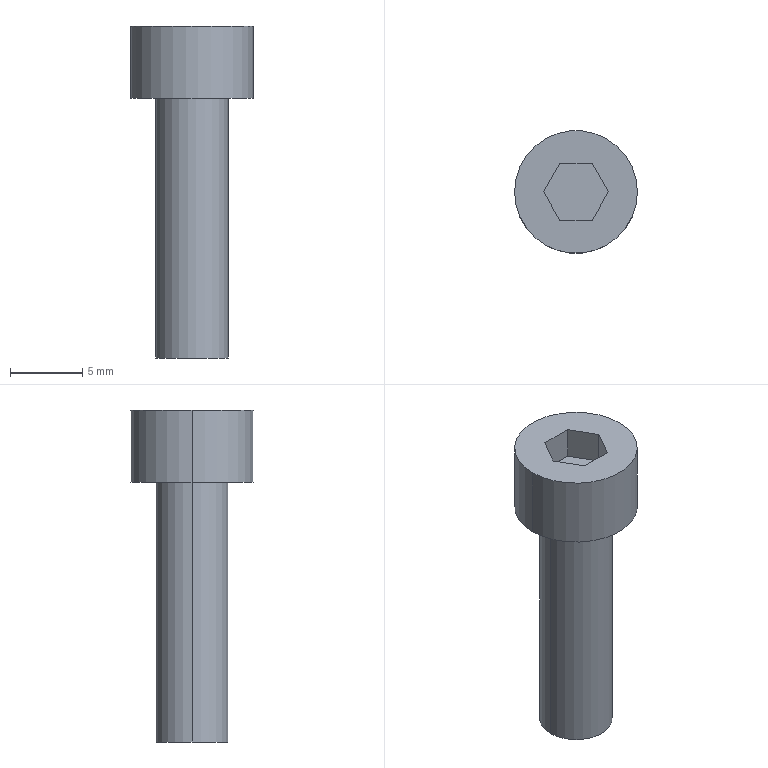Part | SolidWorks | features BaseBody 1 | 1 solid | 14 faces | box 8.5 x 8.5 x 23 mm | volume 607.561 mm3 | plane 10 | cylinder 4 | commonest cylinder face diameters 5 x2 8.5 x2
STEP:
#1=CARTESIAN_POINT('',(2.5,0.,-18.));
#2=VERTEX_POINT('',#1);
#3=CARTESIAN_POINT('',(-2.5,0.,-18.));
#4=VERTEX_POINT('',#3);
#5=CARTESIAN_POINT('',(0.,0.,-18.));
#6=DIRECTION('',(0.,0.,1.));
#7=DIRECTION('',(1.,0.,0.));
#8=AXIS2_PLACEMENT_3D('',#5,#6,#7);
#9=CIRCLE('',#8,2.5);
#10=EDGE_CURVE('',#2,#4,#9,.T.);
#11=ORIENTED_EDGE('',*,*,#10,.T.);
#12=CARTESIAN_POINT('',(-2.5,0.,0.));
#13=VERTEX_POINT('',#12);
#14=CARTESIAN_POINT('',(-2.5,0.,-18.));
#15=DIRECTION('',(0.,0.,1.));
#16=VECTOR('',#15,1000.);
#17=LINE('',#14,#16);
#18=EDGE_CURVE('',#4,#13,#17,.T.);
#19=ORIENTED_EDGE('',*,*,#18,.T.);
#20=CARTESIAN_POINT('',(2.5,0.,0.));
#21=VERTEX_POINT('',#20);
#22=CARTESIAN_POINT('',(0.,0.,0.));
#23=DIRECTION('',(0.,0.,-1.));
#24=DIRECTION('',(1.,0.,0.));
#25=AXIS2_PLACEMENT_3D('',#22,#23,#24);
#26=CIRCLE('',#25,2.5);
#27=EDGE_CURVE('',#13,#21,#26,.T.);
#28=ORIENTED_EDGE('',*,*,#27,.T.);
#29=CARTESIAN_POINT('',(2.5,0.,-18.));
#30=DIRECTION('',(0.,0.,1.));
#31=VECTOR('',#30,1000.);
#32=LINE('',#29,#31);
#33=EDGE_CURVE('',#2,#21,#32,.T.);
#34=ORIENTED_EDGE('',*,*,#33,.F.);
#35=EDGE_LOOP('',(#11,#19,#28,#34));
#36=FACE_OUTER_BOUND('',#35,.T.);
#37=CARTESIAN_POINT('',(0.,0.,-18.));
#38=DIRECTION('',(0.,0.,1.));
#39=DIRECTION('',(1.,0.,0.));
#40=AXIS2_PLACEMENT_3D('',#37,#38,#39);
#41=CYLINDRICAL_SURFACE('',#40,2.5);
#42=ADVANCED_FACE('',(#36),#41,.T.);
#43=CARTESIAN_POINT('',(4.25,0.,0.));
#44=VERTEX_POINT('',#43);
#45=CARTESIAN_POINT('',(-4.25,0.,0.));
#46=VERTEX_POINT('',#45);
#47=CARTESIAN_POINT('',(0.,0.,0.));
#48=DIRECTION('',(0.,0.,1.));
#49=DIRECTION('',(1.,0.,0.));
#50=AXIS2_PLACEMENT_3D('',#47,#48,#49);
#51=CIRCLE('',#50,4.25);
#52=EDGE_CURVE('',#44,#46,#51,.T.);
#53=ORIENTED_EDGE('',*,*,#52,.T.);
#54=CARTESIAN_POINT('',(-4.25,0.,5.));
#55=VERTEX_POINT('',#54);
#56=CARTESIAN_POINT('',(-4.25,0.,0.));
#57=DIRECTION('',(0.,0.,1.));
#58=VECTOR('',#57,1000.);
#59=LINE('',#56,#58);
#60=EDGE_CURVE('',#46,#55,#59,.T.);
#61=ORIENTED_EDGE('',*,*,#60,.T.);
#62=CARTESIAN_POINT('',(4.25,0.,5.));
#63=VERTEX_POINT('',#62);
#64=CARTESIAN_POINT('',(0.,0.,5.));
#65=DIRECTION('',(0.,0.,-1.));
#66=DIRECTION('',(1.,0.,0.));
#67=AXIS2_PLACEMENT_3D('',#64,#65,#66);
#68=CIRCLE('',#67,4.25);
#69=EDGE_CURVE('',#55,#63,#68,.T.);
#70=ORIENTED_EDGE('',*,*,#69,.T.);
#71=CARTESIAN_POINT('',(4.25,0.,0.));
#72=DIRECTION('',(0.,0.,1.));
#73=VECTOR('',#72,1000.);
#74=LINE('',#71,#73);
#75=EDGE_CURVE('',#44,#63,#74,.T.);
#76=ORIENTED_EDGE('',*,*,#75,.F.);
#77=EDGE_LOOP('',(#53,#61,#70,#76));
#78=FACE_OUTER_BOUND('',#77,.T.);
#79=CARTESIAN_POINT('',(0.,0.,0.));
#80=DIRECTION('',(0.,0.,1.));
#81=DIRECTION('',(1.,0.,0.));
#82=AXIS2_PLACEMENT_3D('',#79,#80,#81);
#83=CYLINDRICAL_SURFACE('',#82,4.25);
#84=ADVANCED_FACE('',(#78),#83,.T.);
#85=ORIENTED_EDGE('',*,*,#18,.F.);
#86=CARTESIAN_POINT('',(0.,0.,-18.));
#87=DIRECTION('',(0.,0.,1.));
#88=DIRECTION('',(1.,0.,0.));
#89=AXIS2_PLACEMENT_3D('',#86,#87,#88);
#90=CIRCLE('',#89,2.5);
#91=EDGE_CURVE('',#4,#2,#90,.T.);
#92=ORIENTED_EDGE('',*,*,#91,.T.);
#93=ORIENTED_EDGE('',*,*,#33,.T.);
#94=CARTESIAN_POINT('',(0.,0.,0.));
#95=DIRECTION('',(0.,0.,-1.));
#96=DIRECTION('',(1.,0.,0.));
#97=AXIS2_PLACEMENT_3D('',#94,#95,#96);
#98=CIRCLE('',#97,2.5);
#99=EDGE_CURVE('',#21,#13,#98,.T.);
#100=ORIENTED_EDGE('',*,*,#99,.T.);
#101=EDGE_LOOP('',(#85,#92,#93,#100));
#102=FACE_OUTER_BOUND('',#101,.T.);
#103=CARTESIAN_POINT('',(0.,0.,-18.));
#104=DIRECTION('',(0.,0.,1.));
#105=DIRECTION('',(1.,0.,0.));
#106=AXIS2_PLACEMENT_3D('',#103,#104,#105);
#107=CYLINDRICAL_SURFACE('',#106,2.5);
#108=ADVANCED_FACE('',(#102),#107,.T.);
#109=ORIENTED_EDGE('',*,*,#10,.F.);
#110=ORIENTED_EDGE('',*,*,#91,.F.);
#111=EDGE_LOOP('',(#109,#110));
#112=FACE_OUTER_BOUND('',#111,.T.);
#113=CARTESIAN_POINT('',(0.,0.,-18.));
#114=DIRECTION('',(0.,0.,1.));
#115=DIRECTION('',(1.,0.,0.));
#116=AXIS2_PLACEMENT_3D('',#113,#114,#115);
#117=PLANE('',#116);
#118=ADVANCED_FACE('',(#112),#117,.F.);
#119=ORIENTED_EDGE('',*,*,#99,.F.);
#120=ORIENTED_EDGE('',*,*,#27,.F.);
#121=EDGE_LOOP('',(#119,#120));
#122=FACE_BOUND('',#121,.T.);
#123=ORIENTED_EDGE('',*,*,#52,.F.);
#124=CARTESIAN_POINT('',(0.,0.,0.));
#125=DIRECTION('',(0.,0.,1.));
#126=DIRECTION('',(1.,0.,0.));
#127=AXIS2_PLACEMENT_3D('',#124,#125,#126);
#128=CIRCLE('',#127,4.25);
#129=EDGE_CURVE('',#46,#44,#128,.T.);
#130=ORIENTED_EDGE('',*,*,#129,.F.);
#131=EDGE_LOOP('',(#123,#130));
#132=FACE_OUTER_BOUND('',#131,.T.);
#133=CARTESIAN_POINT('',(0.,0.,0.));
#134=DIRECTION('',(0.,0.,1.));
#135=DIRECTION('',(1.,0.,0.));
#136=AXIS2_PLACEMENT_3D('',#133,#134,#135);
#137=PLANE('',#136);
#138=ADVANCED_FACE('',(#122,#132),#137,.F.);
#139=ORIENTED_EDGE('',*,*,#60,.F.);
#140=ORIENTED_EDGE('',*,*,#129,.T.);
#141=ORIENTED_EDGE('',*,*,#75,.T.);
#142=CARTESIAN_POINT('',(0.,0.,5.));
#143=DIRECTION('',(0.,0.,-1.));
#144=DIRECTION('',(1.,0.,0.));
#145=AXIS2_PLACEMENT_3D('',#142,#143,#144);
#146=CIRCLE('',#145,4.25);
#147=EDGE_CURVE('',#63,#55,#146,.T.);
#148=ORIENTED_EDGE('',*,*,#147,.T.);
#149=EDGE_LOOP('',(#139,#140,#141,#148));
#150=FACE_OUTER_BOUND('',#149,.T.);
#151=CARTESIAN_POINT('',(0.,0.,0.));
#152=DIRECTION('',(0.,0.,1.));
#153=DIRECTION('',(1.,0.,0.));
#154=AXIS2_PLACEMENT_3D('',#151,#152,#153);
#155=CYLINDRICAL_SURFACE('',#154,4.25);
#156=ADVANCED_FACE('',(#150),#155,.T.);
#157=CARTESIAN_POINT('',(-1.125,-1.949,5.));
#158=VERTEX_POINT('',#157);
#159=CARTESIAN_POINT('',(-2.25,0.,5.));
#160=VERTEX_POINT('',#159);
#161=CARTESIAN_POINT('',(-1.125,-1.949,5.));
#162=DIRECTION('',(-0.5,0.866,0.));
#163=VECTOR('',#162,1000.);
#164=LINE('',#161,#163);
#165=EDGE_CURVE('',#158,#160,#164,.T.);
#166=ORIENTED_EDGE('',*,*,#165,.T.);
#167=CARTESIAN_POINT('',(-1.125,1.949,5.));
#168=VERTEX_POINT('',#167);
#169=CARTESIAN_POINT('',(-2.25,0.,5.));
#170=DIRECTION('',(0.5,0.866,0.));
#171=VECTOR('',#170,1000.);
#172=LINE('',#169,#171);
#173=EDGE_CURVE('',#160,#168,#172,.T.);
#174=ORIENTED_EDGE('',*,*,#173,.T.);
#175=CARTESIAN_POINT('',(1.125,1.949,5.));
#176=VERTEX_POINT('',#175);
#177=CARTESIAN_POINT('',(0.,1.949,5.));
#178=DIRECTION('',(1.,0.,0.));
#179=VECTOR('',#178,1000.);
#180=LINE('',#177,#179);
#181=EDGE_CURVE('',#168,#176,#180,.T.);
#182=ORIENTED_EDGE('',*,*,#181,.T.);
#183=CARTESIAN_POINT('',(2.25,0.,5.));
#184=VERTEX_POINT('',#183);
#185=CARTESIAN_POINT('',(1.125,1.949,5.));
#186=DIRECTION('',(0.5,-0.866,0.));
#187=VECTOR('',#186,1000.);
#188=LINE('',#185,#187);
#189=EDGE_CURVE('',#176,#184,#188,.T.);
#190=ORIENTED_EDGE('',*,*,#189,.T.);
#191=CARTESIAN_POINT('',(1.125,-1.949,5.));
#192=VERTEX_POINT('',#191);
#193=CARTESIAN_POINT('',(2.25,0.,5.));
#194=DIRECTION('',(-0.5,-0.866,0.));
#195=VECTOR('',#194,1000.);
#196=LINE('',#193,#195);
#197=EDGE_CURVE('',#184,#192,#196,.T.);
#198=ORIENTED_EDGE('',*,*,#197,.T.);
#199=CARTESIAN_POINT('',(0.,-1.949,5.));
#200=DIRECTION('',(-1.,0.,0.));
#201=VECTOR('',#200,1000.);
#202=LINE('',#199,#201);
#203=EDGE_CURVE('',#192,#158,#202,.T.);
#204=ORIENTED_EDGE('',*,*,#203,.T.);
#205=EDGE_LOOP('',(#166,#174,#182,#190,#198,#204));
#206=FACE_BOUND('',#205,.T.);
#207=ORIENTED_EDGE('',*,*,#147,.F.);
#208=ORIENTED_EDGE('',*,*,#69,.F.);
#209=EDGE_LOOP('',(#207,#208));
#210=FACE_OUTER_BOUND('',#209,.T.);
#211=CARTESIAN_POINT('',(0.,0.,5.));
#212=DIRECTION('',(0.,0.,1.));
#213=DIRECTION('',(1.,0.,0.));
#214=AXIS2_PLACEMENT_3D('',#211,#212,#213);
#215=PLANE('',#214);
#216=ADVANCED_FACE('',(#206,#210),#215,.T.);
#217=ORIENTED_EDGE('',*,*,#173,.F.);
#218=CARTESIAN_POINT('',(-2.25,0.,2.75));
#219=VERTEX_POINT('',#218);
#220=CARTESIAN_POINT('',(-2.25,0.,2.75));
#221=DIRECTION('',(0.,0.,-1.));
#222=VECTOR('',#221,1000.);
#223=LINE('',#220,#222);
#224=EDGE_CURVE('',#160,#219,#223,.T.);
#225=ORIENTED_EDGE('',*,*,#224,.T.);
#226=CARTESIAN_POINT('',(-1.125,1.949,2.75));
#227=VERTEX_POINT('',#226);
#228=CARTESIAN_POINT('',(-1.125,1.949,2.75));
#229=DIRECTION('',(0.5,0.866,0.));
#230=VECTOR('',#229,1000.);
#231=LINE('',#228,#230);
#232=EDGE_CURVE('',#219,#227,#231,.T.);
#233=ORIENTED_EDGE('',*,*,#232,.T.);
#234=CARTESIAN_POINT('',(-1.125,1.949,2.75));
#235=DIRECTION('',(0.,0.,1.));
#236=VECTOR('',#235,1000.);
#237=LINE('',#234,#236);
#238=EDGE_CURVE('',#227,#168,#237,.T.);
#239=ORIENTED_EDGE('',*,*,#238,.T.);
#240=EDGE_LOOP('',(#217,#225,#233,#239));
#241=FACE_OUTER_BOUND('',#240,.T.);
#242=CARTESIAN_POINT('',(-1.125,1.949,2.75));
#243=DIRECTION('',(0.866,-0.5,0.));
#244=DIRECTION('',(0.5,0.866,0.));
#245=AXIS2_PLACEMENT_3D('',#242,#243,#244);
#246=PLANE('',#245);
#247=ADVANCED_FACE('',(#241),#246,.T.);
#248=ORIENTED_EDGE('',*,*,#165,.F.);
#249=CARTESIAN_POINT('',(-1.125,-1.949,2.75));
#250=VERTEX_POINT('',#249);
#251=CARTESIAN_POINT('',(-1.125,-1.949,2.75));
#252=DIRECTION('',(0.,0.,-1.));
#253=VECTOR('',#252,1000.);
#254=LINE('',#251,#253);
#255=EDGE_CURVE('',#158,#250,#254,.T.);
#256=ORIENTED_EDGE('',*,*,#255,.T.);
#257=CARTESIAN_POINT('',(-2.25,0.,2.75));
#258=DIRECTION('',(-0.5,0.866,0.));
#259=VECTOR('',#258,1000.);
#260=LINE('',#257,#259);
#261=EDGE_CURVE('',#250,#219,#260,.T.);
#262=ORIENTED_EDGE('',*,*,#261,.T.);
#263=ORIENTED_EDGE('',*,*,#224,.F.);
#264=EDGE_LOOP('',(#248,#256,#262,#263));
#265=FACE_OUTER_BOUND('',#264,.T.);
#266=CARTESIAN_POINT('',(-2.25,0.,2.75));
#267=DIRECTION('',(0.866,0.5,0.));
#268=DIRECTION('',(-0.5,0.866,0.));
#269=AXIS2_PLACEMENT_3D('',#266,#267,#268);
#270=PLANE('',#269);
#271=ADVANCED_FACE('',(#265),#270,.T.);
#272=ORIENTED_EDGE('',*,*,#203,.F.);
#273=CARTESIAN_POINT('',(1.125,-1.949,2.75));
#274=VERTEX_POINT('',#273);
#275=CARTESIAN_POINT('',(1.125,-1.949,2.75));
#276=DIRECTION('',(0.,0.,-1.));
#277=VECTOR('',#276,1000.);
#278=LINE('',#275,#277);
#279=EDGE_CURVE('',#192,#274,#278,.T.);
#280=ORIENTED_EDGE('',*,*,#279,.T.);
#281=CARTESIAN_POINT('',(-1.125,-1.949,2.75));
#282=DIRECTION('',(-1.,0.,0.));
#283=VECTOR('',#282,1000.);
#284=LINE('',#281,#283);
#285=EDGE_CURVE('',#274,#250,#284,.T.);
#286=ORIENTED_EDGE('',*,*,#285,.T.);
#287=ORIENTED_EDGE('',*,*,#255,.F.);
#288=EDGE_LOOP('',(#272,#280,#286,#287));
#289=FACE_OUTER_BOUND('',#288,.T.);
#290=CARTESIAN_POINT('',(-1.125,-1.949,2.75));
#291=DIRECTION('',(0.,1.,0.));
#292=DIRECTION('',(-1.,0.,0.));
#293=AXIS2_PLACEMENT_3D('',#290,#291,#292);
#294=PLANE('',#293);
#295=ADVANCED_FACE('',(#289),#294,.T.);
#296=ORIENTED_EDGE('',*,*,#197,.F.);
#297=CARTESIAN_POINT('',(2.25,0.,2.75));
#298=VERTEX_POINT('',#297);
#299=CARTESIAN_POINT('',(2.25,0.,2.75));
#300=DIRECTION('',(0.,0.,-1.));
#301=VECTOR('',#300,1000.);
#302=LINE('',#299,#301);
#303=EDGE_CURVE('',#184,#298,#302,.T.);
#304=ORIENTED_EDGE('',*,*,#303,.T.);
#305=CARTESIAN_POINT('',(1.125,-1.949,2.75));
#306=DIRECTION('',(-0.5,-0.866,0.));
#307=VECTOR('',#306,1000.);
#308=LINE('',#305,#307);
#309=EDGE_CURVE('',#298,#274,#308,.T.);
#310=ORIENTED_EDGE('',*,*,#309,.T.);
#311=ORIENTED_EDGE('',*,*,#279,.F.);
#312=EDGE_LOOP('',(#296,#304,#310,#311));
#313=FACE_OUTER_BOUND('',#312,.T.);
#314=CARTESIAN_POINT('',(1.125,-1.949,2.75));
#315=DIRECTION('',(-0.866,0.5,0.));
#316=DIRECTION('',(-0.5,-0.866,0.));
#317=AXIS2_PLACEMENT_3D('',#314,#315,#316);
#318=PLANE('',#317);
#319=ADVANCED_FACE('',(#313),#318,.T.);
#320=ORIENTED_EDGE('',*,*,#189,.F.);
#321=CARTESIAN_POINT('',(1.125,1.949,2.75));
#322=VERTEX_POINT('',#321);
#323=CARTESIAN_POINT('',(1.125,1.949,2.75));
#324=DIRECTION('',(0.,0.,-1.));
#325=VECTOR('',#324,1000.);
#326=LINE('',#323,#325);
#327=EDGE_CURVE('',#176,#322,#326,.T.);
#328=ORIENTED_EDGE('',*,*,#327,.T.);
#329=CARTESIAN_POINT('',(2.25,0.,2.75));
#330=DIRECTION('',(0.5,-0.866,0.));
#331=VECTOR('',#330,1000.);
#332=LINE('',#329,#331);
#333=EDGE_CURVE('',#322,#298,#332,.T.);
#334=ORIENTED_EDGE('',*,*,#333,.T.);
#335=ORIENTED_EDGE('',*,*,#303,.F.);
#336=EDGE_LOOP('',(#320,#328,#334,#335));
#337=FACE_OUTER_BOUND('',#336,.T.);
#338=CARTESIAN_POINT('',(2.25,0.,2.75));
#339=DIRECTION('',(-0.866,-0.5,0.));
#340=DIRECTION('',(0.5,-0.866,0.));
#341=AXIS2_PLACEMENT_3D('',#338,#339,#340);
#342=PLANE('',#341);
#343=ADVANCED_FACE('',(#337),#342,.T.);
#344=ORIENTED_EDGE('',*,*,#181,.F.);
#345=ORIENTED_EDGE('',*,*,#238,.F.);
#346=CARTESIAN_POINT('',(1.125,1.949,2.75));
#347=DIRECTION('',(1.,0.,0.));
#348=VECTOR('',#347,1000.);
#349=LINE('',#346,#348);
#350=EDGE_CURVE('',#227,#322,#349,.T.);
#351=ORIENTED_EDGE('',*,*,#350,.T.);
#352=ORIENTED_EDGE('',*,*,#327,.F.);
#353=EDGE_LOOP('',(#344,#345,#351,#352));
#354=FACE_OUTER_BOUND('',#353,.T.);
#355=CARTESIAN_POINT('',(1.125,1.949,2.75));
#356=DIRECTION('',(0.,-1.,0.));
#357=DIRECTION('',(1.,0.,0.));
#358=AXIS2_PLACEMENT_3D('',#355,#356,#357);
#359=PLANE('',#358);
#360=ADVANCED_FACE('',(#354),#359,.T.);
#361=ORIENTED_EDGE('',*,*,#285,.F.);
#362=ORIENTED_EDGE('',*,*,#309,.F.);
#363=ORIENTED_EDGE('',*,*,#333,.F.);
#364=ORIENTED_EDGE('',*,*,#350,.F.);
#365=ORIENTED_EDGE('',*,*,#232,.F.);
#366=ORIENTED_EDGE('',*,*,#261,.F.);
#367=EDGE_LOOP('',(#361,#362,#363,#364,#365,#366));
#368=FACE_OUTER_BOUND('',#367,.T.);
#369=CARTESIAN_POINT('',(0.,0.,2.75));
#370=DIRECTION('',(0.,0.,1.));
#371=DIRECTION('',(1.,0.,0.));
#372=AXIS2_PLACEMENT_3D('',#369,#370,#371);
#373=PLANE('',#372);
#374=ADVANCED_FACE('',(#368),#373,.T.);
#375=CLOSED_SHELL('',(#42,#84,#108,#118,#138,#156,#216,#247,#271,#295,#319,#343,#360,#374));
#376=MANIFOLD_SOLID_BREP('',#375);
#377=CARTESIAN_POINT('',(0.,0.,0.));
#378=DIRECTION('',(0.,0.,1.));
#379=DIRECTION('',(1.,0.,0.));
#380=AXIS2_PLACEMENT_3D('',#377,#378,#379);
#381=(LENGTH_UNIT()NAMED_UNIT(*)SI_UNIT(.MILLI.,.METRE.));
#382=UNCERTAINTY_MEASURE_WITH_UNIT(LENGTH_MEASURE(0.00001),#381,'','');
#383=(NAMED_UNIT(*)PLANE_ANGLE_UNIT()SI_UNIT($,.RADIAN.));
#384=(NAMED_UNIT(*)SI_UNIT($,.STERADIAN.)SOLID_ANGLE_UNIT());
#385=(GEOMETRIC_REPRESENTATION_CONTEXT(3)GLOBAL_UNCERTAINTY_ASSIGNED_CONTEXT((#382))GLOBAL_UNIT_ASSIGNED_CONTEXT((#381,#383,#384))REPRESENTATION_CONTEXT('',''));
#386=ADVANCED_BREP_SHAPE_REPRESENTATION('',(#376,#380),#385);